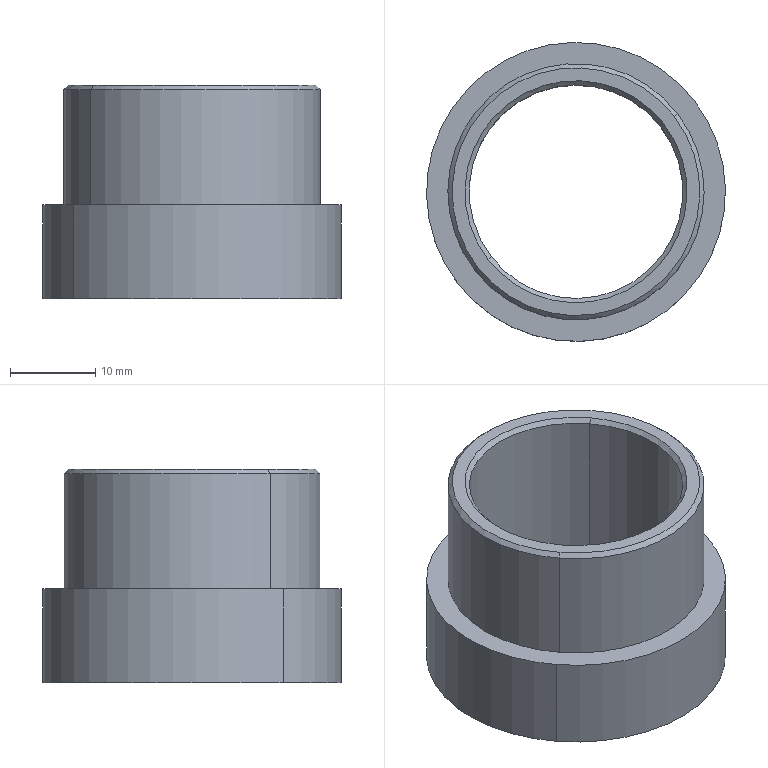Part | NX | features solid 2 | 1 solid | 15 faces | box 35 x 35 x 25 mm | volume 8169 mm3 | cylinder 6 | cone 4 | plane 3 | torus 2 | commonest cylinder face diameters 25 x2 30 x2 35 x2
STEP:
#1=CARTESIAN_POINT('',(-459.908,-1642.621,375.5));
#2=VERTEX_POINT('',#1);
#3=CARTESIAN_POINT('',(-460.305,-1642.925,376.));
#4=VERTEX_POINT('',#3);
#5=CARTESIAN_POINT('',(-460.305,-1642.925,376.));
#6=DIRECTION('',(-0.5605,-0.4311,0.7071));
#7=VECTOR('',#6,1000.);
#8=LINE('',#5,#7);
#9=EDGE_CURVE('',#2,#4,#8,.T.);
#10=ORIENTED_EDGE('',*,*,#9,.F.);
#11=CARTESIAN_POINT('',(-440.092,-1627.379,375.5));
#12=VERTEX_POINT('',#11);
#13=CARTESIAN_POINT('',(-450.,-1635.,375.5));
#14=DIRECTION('',(0.,0.,1.));
#15=DIRECTION('',(0.7927,0.6096,0.));
#16=AXIS2_PLACEMENT_3D('',#13,#14,#15);
#17=CIRCLE('',#16,12.5);
#18=EDGE_CURVE('',#12,#2,#17,.T.);
#19=ORIENTED_EDGE('',*,*,#18,.F.);
#20=CARTESIAN_POINT('',(-439.695,-1627.075,376.));
#21=VERTEX_POINT('',#20);
#22=CARTESIAN_POINT('',(-439.695,-1627.075,376.));
#23=DIRECTION('',(0.5605,0.4311,0.7071));
#24=VECTOR('',#23,1000.);
#25=LINE('',#22,#24);
#26=EDGE_CURVE('',#21,#12,#25,.F.);
#27=ORIENTED_EDGE('',*,*,#26,.F.);
#28=CARTESIAN_POINT('',(-450.,-1635.,376.));
#29=DIRECTION('',(0.,0.,-1.));
#30=DIRECTION('',(0.7927,0.6096,0.));
#31=AXIS2_PLACEMENT_3D('',#28,#29,#30);
#32=CIRCLE('',#31,13.);
#33=EDGE_CURVE('',#4,#21,#32,.T.);
#34=ORIENTED_EDGE('',*,*,#33,.F.);
#35=EDGE_LOOP('',(#10,#19,#27,#34));
#36=FACE_BOUND('',#35,.T.);
#37=CARTESIAN_POINT('',(-450.,-1635.,376.));
#38=DIRECTION('',(0.,0.,1.));
#39=DIRECTION('',(0.7927,0.6096,0.));
#40=AXIS2_PLACEMENT_3D('',#37,#38,#39);
#41=CONICAL_SURFACE('',#40,13.,0.7854);
#42=ADVANCED_FACE('',(#36),#41,.F.);
#43=CARTESIAN_POINT('',(-438.506,-1626.16,376.));
#44=VERTEX_POINT('',#43);
#45=CARTESIAN_POINT('',(-438.11,-1625.855,375.5));
#46=VERTEX_POINT('',#45);
#47=CARTESIAN_POINT('',(-438.11,-1625.855,375.5));
#48=DIRECTION('',(0.5605,0.4311,-0.7071));
#49=VECTOR('',#48,1000.);
#50=LINE('',#47,#49);
#51=EDGE_CURVE('',#44,#46,#50,.T.);
#52=ORIENTED_EDGE('',*,*,#51,.F.);
#53=CARTESIAN_POINT('',(-461.494,-1643.84,376.));
#54=VERTEX_POINT('',#53);
#55=CARTESIAN_POINT('',(-450.,-1635.,376.));
#56=DIRECTION('',(0.,0.,1.));
#57=DIRECTION('',(0.7927,0.6096,0.));
#58=AXIS2_PLACEMENT_3D('',#55,#56,#57);
#59=CIRCLE('',#58,14.5);
#60=EDGE_CURVE('',#54,#44,#59,.T.);
#61=ORIENTED_EDGE('',*,*,#60,.F.);
#62=CARTESIAN_POINT('',(-461.89,-1644.145,375.5));
#63=VERTEX_POINT('',#62);
#64=CARTESIAN_POINT('',(-461.89,-1644.145,375.5));
#65=DIRECTION('',(-0.5605,-0.4311,-0.7071));
#66=VECTOR('',#65,1000.);
#67=LINE('',#64,#66);
#68=EDGE_CURVE('',#63,#54,#67,.F.);
#69=ORIENTED_EDGE('',*,*,#68,.F.);
#70=CARTESIAN_POINT('',(-450.,-1635.,375.5));
#71=DIRECTION('',(0.,0.,-1.));
#72=DIRECTION('',(0.7927,0.6096,0.));
#73=AXIS2_PLACEMENT_3D('',#70,#71,#72);
#74=CIRCLE('',#73,15.);
#75=EDGE_CURVE('',#46,#63,#74,.T.);
#76=ORIENTED_EDGE('',*,*,#75,.F.);
#77=EDGE_LOOP('',(#52,#61,#69,#76));
#78=FACE_BOUND('',#77,.T.);
#79=CARTESIAN_POINT('',(-450.,-1635.,375.5));
#80=DIRECTION('',(0.,0.,-1.));
#81=DIRECTION('',(-0.7927,-0.6096,0.));
#82=AXIS2_PLACEMENT_3D('',#79,#80,#81);
#83=CONICAL_SURFACE('',#82,15.,0.7854);
#84=ADVANCED_FACE('',(#78),#83,.T.);
#85=CARTESIAN_POINT('',(-439.299,-1626.77,351.));
#86=VERTEX_POINT('',#85);
#87=CARTESIAN_POINT('',(-440.092,-1627.379,352.));
#88=VERTEX_POINT('',#87);
#89=CARTESIAN_POINT('',(-439.299,-1626.77,352.));
#90=DIRECTION('',(-0.6096,0.7927,0.));
#91=DIRECTION('',(-0.7927,-0.6096,0.));
#92=AXIS2_PLACEMENT_3D('',#89,#90,#91);
#93=CIRCLE('',#92,1.);
#94=EDGE_CURVE('',#86,#88,#93,.T.);
#95=ORIENTED_EDGE('',*,*,#94,.F.);
#96=CARTESIAN_POINT('',(-460.701,-1643.23,351.));
#97=VERTEX_POINT('',#96);
#98=CARTESIAN_POINT('',(-450.,-1635.,351.));
#99=DIRECTION('',(0.,0.,1.));
#100=DIRECTION('',(-0.7927,-0.6096,0.));
#101=AXIS2_PLACEMENT_3D('',#98,#99,#100);
#102=CIRCLE('',#101,13.5);
#103=EDGE_CURVE('',#97,#86,#102,.T.);
#104=ORIENTED_EDGE('',*,*,#103,.F.);
#105=CARTESIAN_POINT('',(-459.908,-1642.621,352.));
#106=VERTEX_POINT('',#105);
#107=CARTESIAN_POINT('',(-460.701,-1643.23,352.));
#108=DIRECTION('',(0.6096,-0.7927,0.));
#109=DIRECTION('',(0.7927,0.6096,0.));
#110=AXIS2_PLACEMENT_3D('',#107,#108,#109);
#111=CIRCLE('',#110,1.);
#112=EDGE_CURVE('',#106,#97,#111,.F.);
#113=ORIENTED_EDGE('',*,*,#112,.F.);
#114=CARTESIAN_POINT('',(-450.,-1635.,352.));
#115=DIRECTION('',(0.,0.,-1.));
#116=DIRECTION('',(-0.7927,-0.6096,0.));
#117=AXIS2_PLACEMENT_3D('',#114,#115,#116);
#118=CIRCLE('',#117,12.5);
#119=EDGE_CURVE('',#88,#106,#118,.T.);
#120=ORIENTED_EDGE('',*,*,#119,.F.);
#121=EDGE_LOOP('',(#95,#104,#113,#120));
#122=FACE_BOUND('',#121,.T.);
#123=CARTESIAN_POINT('',(-450.,-1635.,352.));
#124=DIRECTION('',(0.,0.,-1.));
#125=DIRECTION('',(-0.7927,-0.6096,0.));
#126=AXIS2_PLACEMENT_3D('',#123,#124,#125);
#127=TOROIDAL_SURFACE('',#126,13.5,1.);
#128=ADVANCED_FACE('',(#122),#127,.T.);
#129=CARTESIAN_POINT('',(-438.11,-1625.855,362.));
#130=VERTEX_POINT('',#129);
#131=CARTESIAN_POINT('',(-438.11,-1625.855,405.));
#132=DIRECTION('',(0.,0.,-1.));
#133=VECTOR('',#132,1000.);
#134=LINE('',#131,#133);
#135=EDGE_CURVE('',#130,#46,#134,.F.);
#136=ORIENTED_EDGE('',*,*,#135,.T.);
#137=ORIENTED_EDGE('',*,*,#75,.T.);
#138=CARTESIAN_POINT('',(-461.89,-1644.145,362.));
#139=VERTEX_POINT('',#138);
#140=CARTESIAN_POINT('',(-461.89,-1644.145,405.));
#141=DIRECTION('',(0.,0.,-1.));
#142=VECTOR('',#141,1000.);
#143=LINE('',#140,#142);
#144=EDGE_CURVE('',#63,#139,#143,.T.);
#145=ORIENTED_EDGE('',*,*,#144,.T.);
#146=CARTESIAN_POINT('',(-450.,-1635.,362.));
#147=DIRECTION('',(0.,0.,-1.));
#148=DIRECTION('',(-0.7927,-0.6096,0.));
#149=AXIS2_PLACEMENT_3D('',#146,#147,#148);
#150=CIRCLE('',#149,15.);
#151=EDGE_CURVE('',#130,#139,#150,.T.);
#152=ORIENTED_EDGE('',*,*,#151,.F.);
#153=EDGE_LOOP('',(#136,#137,#145,#152));
#154=FACE_BOUND('',#153,.T.);
#155=CARTESIAN_POINT('',(-450.,-1635.,405.));
#156=DIRECTION('',(0.,0.,-1.));
#157=DIRECTION('',(-0.7927,-0.6096,0.));
#158=AXIS2_PLACEMENT_3D('',#155,#156,#157);
#159=CYLINDRICAL_SURFACE('',#158,15.);
#160=ADVANCED_FACE('',(#154),#159,.T.);
#161=CARTESIAN_POINT('',(-450.,-1635.,362.));
#162=DIRECTION('',(0.,0.,-1.));
#163=DIRECTION('',(-0.7927,-0.6096,0.));
#164=AXIS2_PLACEMENT_3D('',#161,#162,#163);
#165=CIRCLE('',#164,15.);
#166=EDGE_CURVE('',#139,#130,#165,.T.);
#167=ORIENTED_EDGE('',*,*,#166,.T.);
#168=ORIENTED_EDGE('',*,*,#151,.T.);
#169=EDGE_LOOP('',(#167,#168));
#170=FACE_BOUND('',#169,.T.);
#171=CARTESIAN_POINT('',(-463.872,-1645.669,362.));
#172=VERTEX_POINT('',#171);
#173=CARTESIAN_POINT('',(-436.128,-1624.331,362.));
#174=VERTEX_POINT('',#173);
#175=CARTESIAN_POINT('',(-450.,-1635.,362.));
#176=DIRECTION('',(0.,0.,-1.));
#177=DIRECTION('',(-0.7927,-0.6096,0.));
#178=AXIS2_PLACEMENT_3D('',#175,#176,#177);
#179=CIRCLE('',#178,17.5);
#180=EDGE_CURVE('',#172,#174,#179,.T.);
#181=ORIENTED_EDGE('',*,*,#180,.F.);
#182=CARTESIAN_POINT('',(-450.,-1635.,362.));
#183=DIRECTION('',(0.,0.,-1.));
#184=DIRECTION('',(-0.7927,-0.6096,0.));
#185=AXIS2_PLACEMENT_3D('',#182,#183,#184);
#186=CIRCLE('',#185,17.5);
#187=EDGE_CURVE('',#174,#172,#186,.T.);
#188=ORIENTED_EDGE('',*,*,#187,.F.);
#189=EDGE_LOOP('',(#181,#188));
#190=FACE_BOUND('',#189,.T.);
#191=CARTESIAN_POINT('',(-463.872,-1645.669,362.));
#192=DIRECTION('',(0.,0.,1.));
#193=DIRECTION('',(0.,-1.,0.));
#194=AXIS2_PLACEMENT_3D('',#191,#192,#193);
#195=PLANE('',#194);
#196=ADVANCED_FACE('',(#170,#190),#195,.T.);
#197=CARTESIAN_POINT('',(-436.128,-1624.331,351.));
#198=VERTEX_POINT('',#197);
#199=CARTESIAN_POINT('',(-436.128,-1624.331,405.));
#200=DIRECTION('',(0.,0.,-1.));
#201=VECTOR('',#200,1000.);
#202=LINE('',#199,#201);
#203=EDGE_CURVE('',#174,#198,#202,.T.);
#204=ORIENTED_EDGE('',*,*,#203,.F.);
#205=ORIENTED_EDGE('',*,*,#187,.T.);
#206=CARTESIAN_POINT('',(-463.872,-1645.669,351.));
#207=VERTEX_POINT('',#206);
#208=CARTESIAN_POINT('',(-463.872,-1645.669,405.));
#209=DIRECTION('',(0.,0.,-1.));
#210=VECTOR('',#209,1000.);
#211=LINE('',#208,#210);
#212=EDGE_CURVE('',#207,#172,#211,.F.);
#213=ORIENTED_EDGE('',*,*,#212,.F.);
#214=CARTESIAN_POINT('',(-450.,-1635.,351.));
#215=DIRECTION('',(0.,0.,-1.));
#216=DIRECTION('',(-0.7927,-0.6096,0.));
#217=AXIS2_PLACEMENT_3D('',#214,#215,#216);
#218=CIRCLE('',#217,17.5);
#219=EDGE_CURVE('',#198,#207,#218,.T.);
#220=ORIENTED_EDGE('',*,*,#219,.F.);
#221=EDGE_LOOP('',(#204,#205,#213,#220));
#222=FACE_BOUND('',#221,.T.);
#223=CARTESIAN_POINT('',(-450.,-1635.,405.));
#224=DIRECTION('',(0.,0.,-1.));
#225=DIRECTION('',(-0.7927,-0.6096,0.));
#226=AXIS2_PLACEMENT_3D('',#223,#224,#225);
#227=CYLINDRICAL_SURFACE('',#226,17.5);
#228=ADVANCED_FACE('',(#222),#227,.T.);
#229=ORIENTED_EDGE('',*,*,#103,.T.);
#230=CARTESIAN_POINT('',(-450.,-1635.,351.));
#231=DIRECTION('',(0.,0.,1.));
#232=DIRECTION('',(-0.7927,-0.6096,0.));
#233=AXIS2_PLACEMENT_3D('',#230,#231,#232);
#234=CIRCLE('',#233,13.5);
#235=EDGE_CURVE('',#86,#97,#234,.T.);
#236=ORIENTED_EDGE('',*,*,#235,.T.);
#237=EDGE_LOOP('',(#229,#236));
#238=FACE_BOUND('',#237,.T.);
#239=CARTESIAN_POINT('',(-450.,-1635.,351.));
#240=DIRECTION('',(0.,0.,-1.));
#241=DIRECTION('',(-0.7927,-0.6096,0.));
#242=AXIS2_PLACEMENT_3D('',#239,#240,#241);
#243=CIRCLE('',#242,17.5);
#244=EDGE_CURVE('',#207,#198,#243,.T.);
#245=ORIENTED_EDGE('',*,*,#244,.T.);
#246=ORIENTED_EDGE('',*,*,#219,.T.);
#247=EDGE_LOOP('',(#245,#246));
#248=FACE_BOUND('',#247,.T.);
#249=CARTESIAN_POINT('',(-459.908,-1642.621,351.));
#250=DIRECTION('',(0.,0.,-1.));
#251=DIRECTION('',(0.,-1.,0.));
#252=AXIS2_PLACEMENT_3D('',#249,#250,#251);
#253=PLANE('',#252);
#254=ADVANCED_FACE('',(#238,#248),#253,.T.);
#255=CARTESIAN_POINT('',(-440.092,-1627.379,405.));
#256=DIRECTION('',(0.,0.,-1.));
#257=VECTOR('',#256,1000.);
#258=LINE('',#255,#257);
#259=EDGE_CURVE('',#12,#88,#258,.T.);
#260=ORIENTED_EDGE('',*,*,#259,.F.);
#261=ORIENTED_EDGE('',*,*,#18,.T.);
#262=CARTESIAN_POINT('',(-459.908,-1642.621,405.));
#263=DIRECTION('',(0.,0.,-1.));
#264=VECTOR('',#263,1000.);
#265=LINE('',#262,#264);
#266=EDGE_CURVE('',#106,#2,#265,.F.);
#267=ORIENTED_EDGE('',*,*,#266,.F.);
#268=CARTESIAN_POINT('',(-450.,-1635.,352.));
#269=DIRECTION('',(0.,0.,-1.));
#270=DIRECTION('',(-0.7927,-0.6096,0.));
#271=AXIS2_PLACEMENT_3D('',#268,#269,#270);
#272=CIRCLE('',#271,12.5);
#273=EDGE_CURVE('',#106,#88,#272,.T.);
#274=ORIENTED_EDGE('',*,*,#273,.T.);
#275=EDGE_LOOP('',(#260,#261,#267,#274));
#276=FACE_BOUND('',#275,.T.);
#277=CARTESIAN_POINT('',(-450.,-1635.,405.));
#278=DIRECTION('',(0.,0.,-1.));
#279=DIRECTION('',(-0.7927,-0.6096,0.));
#280=AXIS2_PLACEMENT_3D('',#277,#278,#279);
#281=CYLINDRICAL_SURFACE('',#280,12.5);
#282=ADVANCED_FACE('',(#276),#281,.F.);
#283=CARTESIAN_POINT('',(-450.,-1635.,376.));
#284=DIRECTION('',(0.,0.,-1.));
#285=DIRECTION('',(0.7927,0.6096,0.));
#286=AXIS2_PLACEMENT_3D('',#283,#284,#285);
#287=CIRCLE('',#286,13.);
#288=EDGE_CURVE('',#21,#4,#287,.T.);
#289=ORIENTED_EDGE('',*,*,#288,.T.);
#290=ORIENTED_EDGE('',*,*,#33,.T.);
#291=EDGE_LOOP('',(#289,#290));
#292=FACE_BOUND('',#291,.T.);
#293=ORIENTED_EDGE('',*,*,#60,.T.);
#294=CARTESIAN_POINT('',(-450.,-1635.,376.));
#295=DIRECTION('',(0.,0.,1.));
#296=DIRECTION('',(0.7927,0.6096,0.));
#297=AXIS2_PLACEMENT_3D('',#294,#295,#296);
#298=CIRCLE('',#297,14.5);
#299=EDGE_CURVE('',#44,#54,#298,.T.);
#300=ORIENTED_EDGE('',*,*,#299,.T.);
#301=EDGE_LOOP('',(#293,#300));
#302=FACE_BOUND('',#301,.T.);
#303=CARTESIAN_POINT('',(-461.89,-1644.145,376.));
#304=DIRECTION('',(0.,0.,1.));
#305=DIRECTION('',(0.,-1.,0.));
#306=AXIS2_PLACEMENT_3D('',#303,#304,#305);
#307=PLANE('',#306);
#308=ADVANCED_FACE('',(#292,#302),#307,.T.);
#309=CARTESIAN_POINT('',(-450.,-1635.,375.5));
#310=DIRECTION('',(0.,0.,1.));
#311=DIRECTION('',(0.7927,0.6096,0.));
#312=AXIS2_PLACEMENT_3D('',#309,#310,#311);
#313=CIRCLE('',#312,12.5);
#314=EDGE_CURVE('',#2,#12,#313,.T.);
#315=ORIENTED_EDGE('',*,*,#314,.T.);
#316=ORIENTED_EDGE('',*,*,#259,.T.);
#317=ORIENTED_EDGE('',*,*,#119,.T.);
#318=ORIENTED_EDGE('',*,*,#266,.T.);
#319=EDGE_LOOP('',(#315,#316,#317,#318));
#320=FACE_BOUND('',#319,.T.);
#321=CARTESIAN_POINT('',(-450.,-1635.,405.));
#322=DIRECTION('',(0.,0.,-1.));
#323=DIRECTION('',(-0.7927,-0.6096,0.));
#324=AXIS2_PLACEMENT_3D('',#321,#322,#323);
#325=CYLINDRICAL_SURFACE('',#324,12.5);
#326=ADVANCED_FACE('',(#320),#325,.F.);
#327=ORIENTED_EDGE('',*,*,#180,.T.);
#328=ORIENTED_EDGE('',*,*,#203,.T.);
#329=ORIENTED_EDGE('',*,*,#244,.F.);
#330=ORIENTED_EDGE('',*,*,#212,.T.);
#331=EDGE_LOOP('',(#327,#328,#329,#330));
#332=FACE_BOUND('',#331,.T.);
#333=CARTESIAN_POINT('',(-450.,-1635.,405.));
#334=DIRECTION('',(0.,0.,-1.));
#335=DIRECTION('',(-0.7927,-0.6096,0.));
#336=AXIS2_PLACEMENT_3D('',#333,#334,#335);
#337=CYLINDRICAL_SURFACE('',#336,17.5);
#338=ADVANCED_FACE('',(#332),#337,.T.);
#339=CARTESIAN_POINT('',(-450.,-1635.,375.5));
#340=DIRECTION('',(0.,0.,-1.));
#341=DIRECTION('',(0.7927,0.6096,0.));
#342=AXIS2_PLACEMENT_3D('',#339,#340,#341);
#343=CIRCLE('',#342,15.);
#344=EDGE_CURVE('',#63,#46,#343,.T.);
#345=ORIENTED_EDGE('',*,*,#344,.T.);
#346=ORIENTED_EDGE('',*,*,#135,.F.);
#347=ORIENTED_EDGE('',*,*,#166,.F.);
#348=ORIENTED_EDGE('',*,*,#144,.F.);
#349=EDGE_LOOP('',(#345,#346,#347,#348));
#350=FACE_BOUND('',#349,.T.);
#351=CARTESIAN_POINT('',(-450.,-1635.,405.));
#352=DIRECTION('',(0.,0.,-1.));
#353=DIRECTION('',(-0.7927,-0.6096,0.));
#354=AXIS2_PLACEMENT_3D('',#351,#352,#353);
#355=CYLINDRICAL_SURFACE('',#354,15.);
#356=ADVANCED_FACE('',(#350),#355,.T.);
#357=ORIENTED_EDGE('',*,*,#235,.F.);
#358=ORIENTED_EDGE('',*,*,#94,.T.);
#359=ORIENTED_EDGE('',*,*,#273,.F.);
#360=ORIENTED_EDGE('',*,*,#112,.T.);
#361=EDGE_LOOP('',(#357,#358,#359,#360));
#362=FACE_BOUND('',#361,.T.);
#363=CARTESIAN_POINT('',(-450.,-1635.,352.));
#364=DIRECTION('',(0.,0.,-1.));
#365=DIRECTION('',(-0.7927,-0.6096,0.));
#366=AXIS2_PLACEMENT_3D('',#363,#364,#365);
#367=TOROIDAL_SURFACE('',#366,13.5,1.);
#368=ADVANCED_FACE('',(#362),#367,.T.);
#369=ORIENTED_EDGE('',*,*,#299,.F.);
#370=ORIENTED_EDGE('',*,*,#51,.T.);
#371=ORIENTED_EDGE('',*,*,#344,.F.);
#372=ORIENTED_EDGE('',*,*,#68,.T.);
#373=EDGE_LOOP('',(#369,#370,#371,#372));
#374=FACE_BOUND('',#373,.T.);
#375=CARTESIAN_POINT('',(-450.,-1635.,375.5));
#376=DIRECTION('',(0.,0.,-1.));
#377=DIRECTION('',(-0.7927,-0.6096,0.));
#378=AXIS2_PLACEMENT_3D('',#375,#376,#377);
#379=CONICAL_SURFACE('',#378,15.,0.7854);
#380=ADVANCED_FACE('',(#374),#379,.T.);
#381=ORIENTED_EDGE('',*,*,#314,.F.);
#382=ORIENTED_EDGE('',*,*,#9,.T.);
#383=ORIENTED_EDGE('',*,*,#288,.F.);
#384=ORIENTED_EDGE('',*,*,#26,.T.);
#385=EDGE_LOOP('',(#381,#382,#383,#384));
#386=FACE_BOUND('',#385,.T.);
#387=CARTESIAN_POINT('',(-450.,-1635.,376.));
#388=DIRECTION('',(0.,0.,1.));
#389=DIRECTION('',(0.7927,0.6096,0.));
#390=AXIS2_PLACEMENT_3D('',#387,#388,#389);
#391=CONICAL_SURFACE('',#390,13.,0.7854);
#392=ADVANCED_FACE('',(#386),#391,.F.);
#393=CLOSED_SHELL('',(#42,#84,#128,#160,#196,#228,#254,#282,#308,#326,#338,#356,#368,#380,#392));
#394=MANIFOLD_SOLID_BREP('',#393);
#395=(LENGTH_UNIT()NAMED_UNIT(*)SI_UNIT(.MILLI.,.METRE.));
#396=UNCERTAINTY_MEASURE_WITH_UNIT(LENGTH_MEASURE(0.00001),#395,'','');
#397=(NAMED_UNIT(*)PLANE_ANGLE_UNIT()SI_UNIT($,.RADIAN.));
#398=(NAMED_UNIT(*)SI_UNIT($,.STERADIAN.)SOLID_ANGLE_UNIT());
#399=(GEOMETRIC_REPRESENTATION_CONTEXT(3)GLOBAL_UNCERTAINTY_ASSIGNED_CONTEXT((#396))GLOBAL_UNIT_ASSIGNED_CONTEXT((#395,#397,#398))REPRESENTATION_CONTEXT('',''));
#400=ADVANCED_BREP_SHAPE_REPRESENTATION('',(#394),#399);